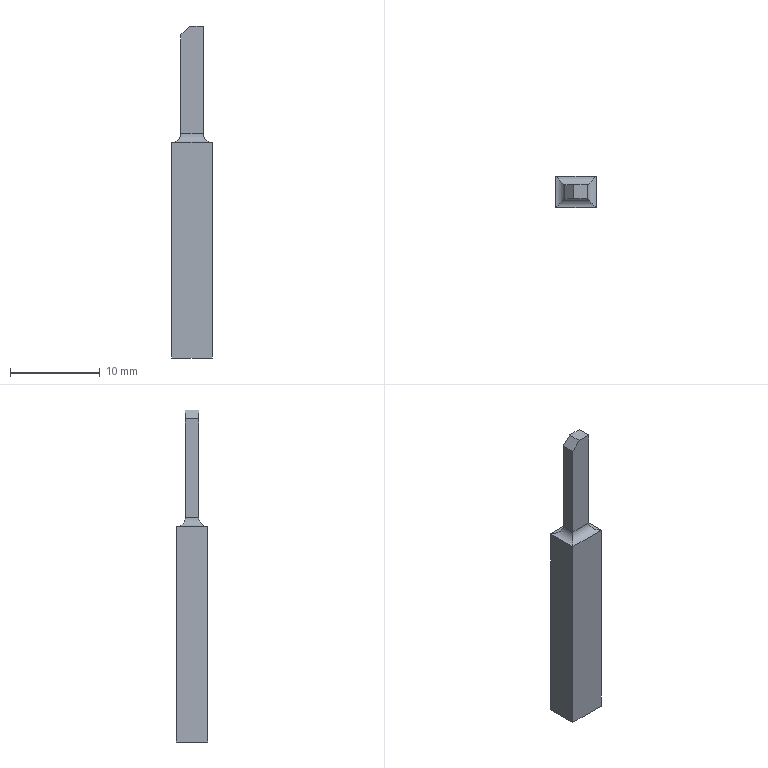Part | STEP file | 03-07 lower cutter | 1 solid | 15 faces | box 4.5 x 3.5 x 37 mm | volume 428.1 mm3 | plane 11 | cylinder 4 | commonest cylinder face diameters 2 x4
STEP:
#1=CARTESIAN_POINT('',(2.25,-1.75,24.));
#2=VERTEX_POINT('',#1);
#3=CARTESIAN_POINT('',(2.25,1.75,24.));
#4=VERTEX_POINT('',#3);
#5=CARTESIAN_POINT('',(2.25,1.75,24.));
#6=DIRECTION('',(0.,1.,0.));
#7=VECTOR('',#6,1000.);
#8=LINE('',#5,#7);
#9=EDGE_CURVE('',#2,#4,#8,.T.);
#10=ORIENTED_EDGE('',*,*,#9,.F.);
#11=CARTESIAN_POINT('',(2.25,-1.75,0.));
#12=VERTEX_POINT('',#11);
#13=CARTESIAN_POINT('',(2.25,-1.75,37.));
#14=DIRECTION('',(0.,0.,-1.));
#15=VECTOR('',#14,1000.);
#16=LINE('',#13,#15);
#17=EDGE_CURVE('',#2,#12,#16,.T.);
#18=ORIENTED_EDGE('',*,*,#17,.T.);
#19=CARTESIAN_POINT('',(2.25,1.75,0.));
#20=VERTEX_POINT('',#19);
#21=CARTESIAN_POINT('',(2.25,1.75,0.));
#22=DIRECTION('',(0.,1.,0.));
#23=VECTOR('',#22,1000.);
#24=LINE('',#21,#23);
#25=EDGE_CURVE('',#12,#20,#24,.T.);
#26=ORIENTED_EDGE('',*,*,#25,.T.);
#27=CARTESIAN_POINT('',(2.25,1.75,37.));
#28=DIRECTION('',(0.,0.,-1.));
#29=VECTOR('',#28,1000.);
#30=LINE('',#27,#29);
#31=EDGE_CURVE('',#4,#20,#30,.T.);
#32=ORIENTED_EDGE('',*,*,#31,.F.);
#33=EDGE_LOOP('',(#10,#18,#26,#32));
#34=FACE_OUTER_BOUND('',#33,.T.);
#35=CARTESIAN_POINT('',(2.25,1.75,37.));
#36=DIRECTION('',(-1.,0.,0.));
#37=DIRECTION('',(0.,-1.,0.));
#38=AXIS2_PLACEMENT_3D('',#35,#36,#37);
#39=PLANE('',#38);
#40=ADVANCED_FACE('',(#34),#39,.F.);
#41=CARTESIAN_POINT('',(-2.25,1.75,24.));
#42=VERTEX_POINT('',#41);
#43=CARTESIAN_POINT('',(-2.25,1.75,24.));
#44=DIRECTION('',(-1.,0.,0.));
#45=VECTOR('',#44,1000.);
#46=LINE('',#43,#45);
#47=EDGE_CURVE('',#4,#42,#46,.T.);
#48=ORIENTED_EDGE('',*,*,#47,.F.);
#49=ORIENTED_EDGE('',*,*,#31,.T.);
#50=CARTESIAN_POINT('',(-2.25,1.75,0.));
#51=VERTEX_POINT('',#50);
#52=CARTESIAN_POINT('',(-2.25,1.75,0.));
#53=DIRECTION('',(-1.,0.,0.));
#54=VECTOR('',#53,1000.);
#55=LINE('',#52,#54);
#56=EDGE_CURVE('',#20,#51,#55,.T.);
#57=ORIENTED_EDGE('',*,*,#56,.T.);
#58=CARTESIAN_POINT('',(-2.25,1.75,37.));
#59=DIRECTION('',(0.,0.,-1.));
#60=VECTOR('',#59,1000.);
#61=LINE('',#58,#60);
#62=EDGE_CURVE('',#42,#51,#61,.T.);
#63=ORIENTED_EDGE('',*,*,#62,.F.);
#64=EDGE_LOOP('',(#48,#49,#57,#63));
#65=FACE_OUTER_BOUND('',#64,.T.);
#66=CARTESIAN_POINT('',(-2.25,1.75,37.));
#67=DIRECTION('',(0.,-1.,0.));
#68=DIRECTION('',(0.,0.,-1.));
#69=AXIS2_PLACEMENT_3D('',#66,#67,#68);
#70=PLANE('',#69);
#71=ADVANCED_FACE('',(#65),#70,.F.);
#72=CARTESIAN_POINT('',(-2.25,-1.75,24.));
#73=VERTEX_POINT('',#72);
#74=CARTESIAN_POINT('',(-2.25,1.75,24.));
#75=DIRECTION('',(0.,-1.,0.));
#76=VECTOR('',#75,1000.);
#77=LINE('',#74,#76);
#78=EDGE_CURVE('',#42,#73,#77,.T.);
#79=ORIENTED_EDGE('',*,*,#78,.F.);
#80=ORIENTED_EDGE('',*,*,#62,.T.);
#81=CARTESIAN_POINT('',(-2.25,-1.75,0.));
#82=VERTEX_POINT('',#81);
#83=CARTESIAN_POINT('',(-2.25,1.75,0.));
#84=DIRECTION('',(0.,-1.,0.));
#85=VECTOR('',#84,1000.);
#86=LINE('',#83,#85);
#87=EDGE_CURVE('',#51,#82,#86,.T.);
#88=ORIENTED_EDGE('',*,*,#87,.T.);
#89=CARTESIAN_POINT('',(-2.25,-1.75,37.));
#90=DIRECTION('',(0.,0.,-1.));
#91=VECTOR('',#90,1000.);
#92=LINE('',#89,#91);
#93=EDGE_CURVE('',#73,#82,#92,.T.);
#94=ORIENTED_EDGE('',*,*,#93,.F.);
#95=EDGE_LOOP('',(#79,#80,#88,#94));
#96=FACE_OUTER_BOUND('',#95,.T.);
#97=CARTESIAN_POINT('',(-2.25,1.75,37.));
#98=DIRECTION('',(1.,0.,0.));
#99=DIRECTION('',(0.,1.,0.));
#100=AXIS2_PLACEMENT_3D('',#97,#98,#99);
#101=PLANE('',#100);
#102=ADVANCED_FACE('',(#96),#101,.F.);
#103=CARTESIAN_POINT('',(-2.25,-1.75,24.));
#104=DIRECTION('',(1.,0.,0.));
#105=VECTOR('',#104,1000.);
#106=LINE('',#103,#105);
#107=EDGE_CURVE('',#73,#2,#106,.T.);
#108=ORIENTED_EDGE('',*,*,#107,.F.);
#109=ORIENTED_EDGE('',*,*,#93,.T.);
#110=CARTESIAN_POINT('',(-2.25,-1.75,0.));
#111=DIRECTION('',(1.,0.,0.));
#112=VECTOR('',#111,1000.);
#113=LINE('',#110,#112);
#114=EDGE_CURVE('',#82,#12,#113,.T.);
#115=ORIENTED_EDGE('',*,*,#114,.T.);
#116=ORIENTED_EDGE('',*,*,#17,.F.);
#117=EDGE_LOOP('',(#108,#109,#115,#116));
#118=FACE_OUTER_BOUND('',#117,.T.);
#119=CARTESIAN_POINT('',(-2.25,-1.75,37.));
#120=DIRECTION('',(0.,1.,0.));
#121=DIRECTION('',(0.,0.,1.));
#122=AXIS2_PLACEMENT_3D('',#119,#120,#121);
#123=PLANE('',#122);
#124=ADVANCED_FACE('',(#118),#123,.F.);
#125=ORIENTED_EDGE('',*,*,#25,.F.);
#126=ORIENTED_EDGE('',*,*,#114,.F.);
#127=ORIENTED_EDGE('',*,*,#87,.F.);
#128=ORIENTED_EDGE('',*,*,#56,.F.);
#129=EDGE_LOOP('',(#125,#126,#127,#128));
#130=FACE_OUTER_BOUND('',#129,.T.);
#131=CARTESIAN_POINT('',(2.25,-1.75,0.));
#132=DIRECTION('',(0.,0.,1.));
#133=DIRECTION('',(1.,0.,0.));
#134=AXIS2_PLACEMENT_3D('',#131,#132,#133);
#135=PLANE('',#134);
#136=ADVANCED_FACE('',(#130),#135,.F.);
#137=CARTESIAN_POINT('',(1.25,-0.75,25.));
#138=VERTEX_POINT('',#137);
#139=CARTESIAN_POINT('',(1.25,-0.75,37.));
#140=VERTEX_POINT('',#139);
#141=CARTESIAN_POINT('',(1.25,-0.75,24.));
#142=DIRECTION('',(0.,0.,1.));
#143=VECTOR('',#142,1000.);
#144=LINE('',#141,#143);
#145=EDGE_CURVE('',#138,#140,#144,.T.);
#146=ORIENTED_EDGE('',*,*,#145,.F.);
#147=CARTESIAN_POINT('',(1.25,0.75,25.));
#148=VERTEX_POINT('',#147);
#149=CARTESIAN_POINT('',(1.25,0.75,25.));
#150=DIRECTION('',(0.,1.,0.));
#151=VECTOR('',#150,1000.);
#152=LINE('',#149,#151);
#153=EDGE_CURVE('',#138,#148,#152,.T.);
#154=ORIENTED_EDGE('',*,*,#153,.T.);
#155=CARTESIAN_POINT('',(1.25,0.75,37.));
#156=VERTEX_POINT('',#155);
#157=CARTESIAN_POINT('',(1.25,0.75,24.));
#158=DIRECTION('',(0.,0.,1.));
#159=VECTOR('',#158,1000.);
#160=LINE('',#157,#159);
#161=EDGE_CURVE('',#148,#156,#160,.T.);
#162=ORIENTED_EDGE('',*,*,#161,.T.);
#163=CARTESIAN_POINT('',(1.25,0.75,37.));
#164=DIRECTION('',(0.,1.,0.));
#165=VECTOR('',#164,1000.);
#166=LINE('',#163,#165);
#167=EDGE_CURVE('',#140,#156,#166,.T.);
#168=ORIENTED_EDGE('',*,*,#167,.F.);
#169=EDGE_LOOP('',(#146,#154,#162,#168));
#170=FACE_OUTER_BOUND('',#169,.T.);
#171=CARTESIAN_POINT('',(1.25,0.75,24.));
#172=DIRECTION('',(1.,0.,0.));
#173=DIRECTION('',(0.,0.,-1.));
#174=AXIS2_PLACEMENT_3D('',#171,#172,#173);
#175=PLANE('',#174);
#176=ADVANCED_FACE('',(#170),#175,.T.);
#177=CARTESIAN_POINT('',(-1.25,-0.75,36.));
#178=VERTEX_POINT('',#177);
#179=CARTESIAN_POINT('',(-0.25,-0.75,37.));
#180=VERTEX_POINT('',#179);
#181=CARTESIAN_POINT('',(-7.25,-0.75,30.));
#182=DIRECTION('',(0.7071,0.,0.7071));
#183=VECTOR('',#182,1000.);
#184=LINE('',#181,#183);
#185=EDGE_CURVE('',#178,#180,#184,.T.);
#186=ORIENTED_EDGE('',*,*,#185,.F.);
#187=CARTESIAN_POINT('',(-1.25,-0.75,25.));
#188=VERTEX_POINT('',#187);
#189=CARTESIAN_POINT('',(-1.25,-0.75,24.));
#190=DIRECTION('',(0.,0.,1.));
#191=VECTOR('',#190,1000.);
#192=LINE('',#189,#191);
#193=EDGE_CURVE('',#188,#178,#192,.T.);
#194=ORIENTED_EDGE('',*,*,#193,.F.);
#195=CARTESIAN_POINT('',(1.25,-0.75,25.));
#196=DIRECTION('',(1.,0.,0.));
#197=VECTOR('',#196,1000.);
#198=LINE('',#195,#197);
#199=EDGE_CURVE('',#188,#138,#198,.T.);
#200=ORIENTED_EDGE('',*,*,#199,.T.);
#201=ORIENTED_EDGE('',*,*,#145,.T.);
#202=CARTESIAN_POINT('',(-1.25,-0.75,37.));
#203=DIRECTION('',(1.,0.,0.));
#204=VECTOR('',#203,1000.);
#205=LINE('',#202,#204);
#206=EDGE_CURVE('',#180,#140,#205,.T.);
#207=ORIENTED_EDGE('',*,*,#206,.F.);
#208=EDGE_LOOP('',(#186,#194,#200,#201,#207));
#209=FACE_OUTER_BOUND('',#208,.T.);
#210=CARTESIAN_POINT('',(-1.25,-0.75,24.));
#211=DIRECTION('',(0.,-1.,0.));
#212=DIRECTION('',(0.,0.,-1.));
#213=AXIS2_PLACEMENT_3D('',#210,#211,#212);
#214=PLANE('',#213);
#215=ADVANCED_FACE('',(#209),#214,.T.);
#216=CARTESIAN_POINT('',(-1.25,0.75,36.));
#217=VERTEX_POINT('',#216);
#218=CARTESIAN_POINT('',(-1.25,-14.25,36.));
#219=DIRECTION('',(0.,1.,0.));
#220=VECTOR('',#219,1000.);
#221=LINE('',#218,#220);
#222=EDGE_CURVE('',#178,#217,#221,.T.);
#223=ORIENTED_EDGE('',*,*,#222,.T.);
#224=CARTESIAN_POINT('',(-1.25,0.75,25.));
#225=VERTEX_POINT('',#224);
#226=CARTESIAN_POINT('',(-1.25,0.75,24.));
#227=DIRECTION('',(0.,0.,1.));
#228=VECTOR('',#227,1000.);
#229=LINE('',#226,#228);
#230=EDGE_CURVE('',#225,#217,#229,.T.);
#231=ORIENTED_EDGE('',*,*,#230,.F.);
#232=CARTESIAN_POINT('',(-1.25,-0.75,25.));
#233=DIRECTION('',(0.,-1.,0.));
#234=VECTOR('',#233,1000.);
#235=LINE('',#232,#234);
#236=EDGE_CURVE('',#225,#188,#235,.T.);
#237=ORIENTED_EDGE('',*,*,#236,.T.);
#238=ORIENTED_EDGE('',*,*,#193,.T.);
#239=EDGE_LOOP('',(#223,#231,#237,#238));
#240=FACE_OUTER_BOUND('',#239,.T.);
#241=CARTESIAN_POINT('',(-1.25,0.75,24.));
#242=DIRECTION('',(-1.,0.,0.));
#243=DIRECTION('',(0.,-1.,0.));
#244=AXIS2_PLACEMENT_3D('',#241,#242,#243);
#245=PLANE('',#244);
#246=ADVANCED_FACE('',(#240),#245,.T.);
#247=CARTESIAN_POINT('',(-0.25,0.75,37.));
#248=VERTEX_POINT('',#247);
#249=CARTESIAN_POINT('',(-0.25,0.75,37.));
#250=DIRECTION('',(-0.7071,0.,-0.7071));
#251=VECTOR('',#250,1000.);
#252=LINE('',#249,#251);
#253=EDGE_CURVE('',#248,#217,#252,.T.);
#254=ORIENTED_EDGE('',*,*,#253,.F.);
#255=CARTESIAN_POINT('',(-1.25,0.75,37.));
#256=DIRECTION('',(-1.,0.,0.));
#257=VECTOR('',#256,1000.);
#258=LINE('',#255,#257);
#259=EDGE_CURVE('',#156,#248,#258,.T.);
#260=ORIENTED_EDGE('',*,*,#259,.F.);
#261=ORIENTED_EDGE('',*,*,#161,.F.);
#262=CARTESIAN_POINT('',(-1.25,0.75,25.));
#263=DIRECTION('',(-1.,0.,0.));
#264=VECTOR('',#263,1000.);
#265=LINE('',#262,#264);
#266=EDGE_CURVE('',#148,#225,#265,.T.);
#267=ORIENTED_EDGE('',*,*,#266,.T.);
#268=ORIENTED_EDGE('',*,*,#230,.T.);
#269=EDGE_LOOP('',(#254,#260,#261,#267,#268));
#270=FACE_OUTER_BOUND('',#269,.T.);
#271=CARTESIAN_POINT('',(-1.25,0.75,24.));
#272=DIRECTION('',(0.,1.,0.));
#273=DIRECTION('',(0.,0.,1.));
#274=AXIS2_PLACEMENT_3D('',#271,#272,#273);
#275=PLANE('',#274);
#276=ADVANCED_FACE('',(#270),#275,.T.);
#277=CARTESIAN_POINT('',(-0.25,-1.75,37.));
#278=DIRECTION('',(0.,1.,0.));
#279=VECTOR('',#278,1000.);
#280=LINE('',#277,#279);
#281=EDGE_CURVE('',#180,#248,#280,.T.);
#282=ORIENTED_EDGE('',*,*,#281,.F.);
#283=ORIENTED_EDGE('',*,*,#206,.T.);
#284=ORIENTED_EDGE('',*,*,#167,.T.);
#285=ORIENTED_EDGE('',*,*,#259,.T.);
#286=EDGE_LOOP('',(#282,#283,#284,#285));
#287=FACE_OUTER_BOUND('',#286,.T.);
#288=CARTESIAN_POINT('',(2.25,-1.75,37.));
#289=DIRECTION('',(0.,0.,1.));
#290=DIRECTION('',(1.,0.,0.));
#291=AXIS2_PLACEMENT_3D('',#288,#289,#290);
#292=PLANE('',#291);
#293=ADVANCED_FACE('',(#287),#292,.T.);
#294=CARTESIAN_POINT('',(-2.25,1.75,24.));
#295=CARTESIAN_POINT('',(-1.664,1.164,24.));
#296=CARTESIAN_POINT('',(-1.25,0.75,24.414));
#297=CARTESIAN_POINT('',(-1.25,0.75,25.));
#298=(BOUNDED_CURVE()B_SPLINE_CURVE(3,(#294,#295,#296,#297),.UNSPECIFIED.,.F.,.F.)B_SPLINE_CURVE_WITH_KNOTS((4,4),(4.712,6.283),.UNSPECIFIED.)CURVE()GEOMETRIC_REPRESENTATION_ITEM()RATIONAL_B_SPLINE_CURVE((1.,0.8047,0.8047,1.))REPRESENTATION_ITEM(''));
#299=EDGE_CURVE('',#42,#225,#298,.T.);
#300=ORIENTED_EDGE('',*,*,#299,.F.);
#301=ORIENTED_EDGE('',*,*,#78,.T.);
#302=CARTESIAN_POINT('',(-1.25,-0.75,25.));
#303=CARTESIAN_POINT('',(-1.25,-0.75,24.414));
#304=CARTESIAN_POINT('',(-1.664,-1.164,24.));
#305=CARTESIAN_POINT('',(-2.25,-1.75,24.));
#306=(BOUNDED_CURVE()B_SPLINE_CURVE(3,(#302,#303,#304,#305),.UNSPECIFIED.,.F.,.F.)B_SPLINE_CURVE_WITH_KNOTS((4,4),(0.,1.571),.UNSPECIFIED.)CURVE()GEOMETRIC_REPRESENTATION_ITEM()RATIONAL_B_SPLINE_CURVE((1.,0.8047,0.8047,1.))REPRESENTATION_ITEM(''));
#307=EDGE_CURVE('',#188,#73,#306,.T.);
#308=ORIENTED_EDGE('',*,*,#307,.F.);
#309=ORIENTED_EDGE('',*,*,#236,.F.);
#310=EDGE_LOOP('',(#300,#301,#308,#309));
#311=FACE_OUTER_BOUND('',#310,.T.);
#312=CARTESIAN_POINT('',(-2.25,0.75,25.));
#313=DIRECTION('',(0.,1.,0.));
#314=DIRECTION('',(-1.,0.,0.));
#315=AXIS2_PLACEMENT_3D('',#312,#313,#314);
#316=CYLINDRICAL_SURFACE('',#315,1.);
#317=ADVANCED_FACE('',(#311),#316,.F.);
#318=ORIENTED_EDGE('',*,*,#307,.T.);
#319=ORIENTED_EDGE('',*,*,#107,.T.);
#320=CARTESIAN_POINT('',(1.25,-0.75,25.));
#321=CARTESIAN_POINT('',(1.25,-0.75,24.414));
#322=CARTESIAN_POINT('',(1.664,-1.164,24.));
#323=CARTESIAN_POINT('',(2.25,-1.75,24.));
#324=(BOUNDED_CURVE()B_SPLINE_CURVE(3,(#320,#321,#322,#323),.UNSPECIFIED.,.F.,.F.)B_SPLINE_CURVE_WITH_KNOTS((4,4),(0.,1.571),.UNSPECIFIED.)CURVE()GEOMETRIC_REPRESENTATION_ITEM()RATIONAL_B_SPLINE_CURVE((1.,0.8047,0.8047,1.))REPRESENTATION_ITEM(''));
#325=EDGE_CURVE('',#138,#2,#324,.T.);
#326=ORIENTED_EDGE('',*,*,#325,.F.);
#327=ORIENTED_EDGE('',*,*,#199,.F.);
#328=EDGE_LOOP('',(#318,#319,#326,#327));
#329=FACE_OUTER_BOUND('',#328,.T.);
#330=CARTESIAN_POINT('',(-1.25,-1.75,25.));
#331=DIRECTION('',(-1.,0.,0.));
#332=DIRECTION('',(0.,0.,1.));
#333=AXIS2_PLACEMENT_3D('',#330,#331,#332);
#334=CYLINDRICAL_SURFACE('',#333,1.);
#335=ADVANCED_FACE('',(#329),#334,.F.);
#336=ORIENTED_EDGE('',*,*,#299,.T.);
#337=ORIENTED_EDGE('',*,*,#266,.F.);
#338=CARTESIAN_POINT('',(2.25,1.75,24.));
#339=CARTESIAN_POINT('',(1.664,1.164,24.));
#340=CARTESIAN_POINT('',(1.25,0.75,24.414));
#341=CARTESIAN_POINT('',(1.25,0.75,25.));
#342=(BOUNDED_CURVE()B_SPLINE_CURVE(3,(#338,#339,#340,#341),.UNSPECIFIED.,.F.,.F.)B_SPLINE_CURVE_WITH_KNOTS((4,4),(1.571,3.142),.UNSPECIFIED.)CURVE()GEOMETRIC_REPRESENTATION_ITEM()RATIONAL_B_SPLINE_CURVE((1.,0.8047,0.8047,1.))REPRESENTATION_ITEM(''));
#343=EDGE_CURVE('',#4,#148,#342,.T.);
#344=ORIENTED_EDGE('',*,*,#343,.F.);
#345=ORIENTED_EDGE('',*,*,#47,.T.);
#346=EDGE_LOOP('',(#336,#337,#344,#345));
#347=FACE_OUTER_BOUND('',#346,.T.);
#348=CARTESIAN_POINT('',(-1.25,1.75,25.));
#349=DIRECTION('',(1.,0.,0.));
#350=DIRECTION('',(0.,0.,-1.));
#351=AXIS2_PLACEMENT_3D('',#348,#349,#350);
#352=CYLINDRICAL_SURFACE('',#351,1.);
#353=ADVANCED_FACE('',(#347),#352,.F.);
#354=ORIENTED_EDGE('',*,*,#325,.T.);
#355=ORIENTED_EDGE('',*,*,#9,.T.);
#356=ORIENTED_EDGE('',*,*,#343,.T.);
#357=ORIENTED_EDGE('',*,*,#153,.F.);
#358=EDGE_LOOP('',(#354,#355,#356,#357));
#359=FACE_OUTER_BOUND('',#358,.T.);
#360=CARTESIAN_POINT('',(2.25,0.75,25.));
#361=DIRECTION('',(0.,-1.,0.));
#362=DIRECTION('',(0.,0.,-1.));
#363=AXIS2_PLACEMENT_3D('',#360,#361,#362);
#364=CYLINDRICAL_SURFACE('',#363,1.);
#365=ADVANCED_FACE('',(#359),#364,.F.);
#366=ORIENTED_EDGE('',*,*,#185,.T.);
#367=ORIENTED_EDGE('',*,*,#281,.T.);
#368=ORIENTED_EDGE('',*,*,#253,.T.);
#369=ORIENTED_EDGE('',*,*,#222,.F.);
#370=EDGE_LOOP('',(#366,#367,#368,#369));
#371=FACE_OUTER_BOUND('',#370,.T.);
#372=CARTESIAN_POINT('',(-0.25,-14.25,37.));
#373=DIRECTION('',(0.7071,0.,-0.7071));
#374=DIRECTION('',(-0.7071,0.,-0.7071));
#375=AXIS2_PLACEMENT_3D('',#372,#373,#374);
#376=PLANE('',#375);
#377=ADVANCED_FACE('',(#371),#376,.F.);
#378=CLOSED_SHELL('',(#40,#71,#102,#124,#136,#176,#215,#246,#276,#293,#317,#335,#353,#365,#377));
#379=MANIFOLD_SOLID_BREP('',#378);
#380=CARTESIAN_POINT('',(0.,0.,0.));
#381=DIRECTION('',(0.,0.,1.));
#382=DIRECTION('',(1.,0.,0.));
#383=AXIS2_PLACEMENT_3D('',#380,#381,#382);
#384=(LENGTH_UNIT()NAMED_UNIT(*)SI_UNIT(.MILLI.,.METRE.));
#385=UNCERTAINTY_MEASURE_WITH_UNIT(LENGTH_MEASURE(0.00001),#384,'','');
#386=(NAMED_UNIT(*)PLANE_ANGLE_UNIT()SI_UNIT($,.RADIAN.));
#387=(NAMED_UNIT(*)SI_UNIT($,.STERADIAN.)SOLID_ANGLE_UNIT());
#388=(GEOMETRIC_REPRESENTATION_CONTEXT(3)GLOBAL_UNCERTAINTY_ASSIGNED_CONTEXT((#385))GLOBAL_UNIT_ASSIGNED_CONTEXT((#384,#386,#387))REPRESENTATION_CONTEXT('',''));
#389=ADVANCED_BREP_SHAPE_REPRESENTATION('',(#379,#383),#388);